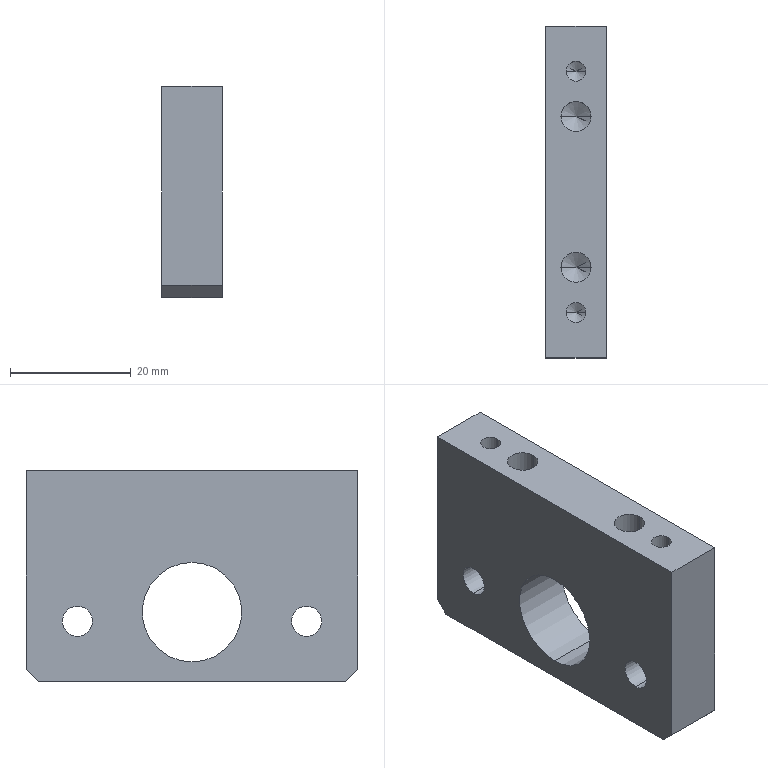Part | SolidWorks | features HoleWzd 3, Chamfer 1, Extrusion 1, ICE 1, MirrorPattern 1 | 1 solid | 30 faces | box 10 x 55 x 35 mm | volume 16084 mm3 | cylinder 14 | cone 8 | plane 8 | commonest cylinder face diameters 5 x8 3.3 x4 16.5 x2
STEP:
#1=CARTESIAN_POINT('',(2.5,12.5,7.4));
#2=VERTEX_POINT('',#1);
#3=CARTESIAN_POINT('',(7.5,12.5,7.4));
#4=VERTEX_POINT('',#3);
#5=CARTESIAN_POINT('',(5.,12.5,7.4));
#6=DIRECTION('',(0.,0.,1.));
#7=DIRECTION('',(1.,0.,0.));
#8=AXIS2_PLACEMENT_3D('',#5,#6,#7);
#9=CIRCLE('',#8,2.5);
#10=EDGE_CURVE('',#2,#4,#9,.T.);
#11=ORIENTED_EDGE('',*,*,#10,.F.);
#12=CARTESIAN_POINT('',(2.5,12.5,17.5));
#13=VERTEX_POINT('',#12);
#14=CARTESIAN_POINT('',(2.5,12.5,17.5));
#15=DIRECTION('',(0.,0.,1.));
#16=VECTOR('',#15,1000.);
#17=LINE('',#14,#16);
#18=EDGE_CURVE('',#2,#13,#17,.T.);
#19=ORIENTED_EDGE('',*,*,#18,.T.);
#20=CARTESIAN_POINT('',(7.5,12.5,17.5));
#21=VERTEX_POINT('',#20);
#22=CARTESIAN_POINT('',(5.,12.5,17.5));
#23=DIRECTION('',(0.,0.,1.));
#24=DIRECTION('',(1.,0.,0.));
#25=AXIS2_PLACEMENT_3D('',#22,#23,#24);
#26=CIRCLE('',#25,2.5);
#27=EDGE_CURVE('',#13,#21,#26,.T.);
#28=ORIENTED_EDGE('',*,*,#27,.T.);
#29=CARTESIAN_POINT('',(7.5,12.5,17.5));
#30=DIRECTION('',(0.,0.,1.));
#31=VECTOR('',#30,1000.);
#32=LINE('',#29,#31);
#33=EDGE_CURVE('',#4,#21,#32,.T.);
#34=ORIENTED_EDGE('',*,*,#33,.F.);
#35=EDGE_LOOP('',(#11,#19,#28,#34));
#36=FACE_OUTER_BOUND('',#35,.T.);
#37=CARTESIAN_POINT('',(5.,12.5,17.5));
#38=DIRECTION('',(0.,0.,1.));
#39=DIRECTION('',(1.,0.,0.));
#40=AXIS2_PLACEMENT_3D('',#37,#38,#39);
#41=CYLINDRICAL_SURFACE('',#40,2.5);
#42=ADVANCED_FACE('',(#36),#41,.F.);
#43=CARTESIAN_POINT('',(5.,12.5,5.898));
#44=VERTEX_POINT('',#43);
#45=CARTESIAN_POINT('',(7.5,12.5,7.4));
#46=DIRECTION('',(0.8572,0.,0.515));
#47=VECTOR('',#46,1000.);
#48=LINE('',#45,#47);
#49=EDGE_CURVE('',#44,#4,#48,.T.);
#50=ORIENTED_EDGE('',*,*,#49,.F.);
#51=CARTESIAN_POINT('',(2.5,12.5,7.4));
#52=DIRECTION('',(-0.8572,0.,0.515));
#53=VECTOR('',#52,1000.);
#54=LINE('',#51,#53);
#55=EDGE_CURVE('',#44,#2,#54,.T.);
#56=ORIENTED_EDGE('',*,*,#55,.T.);
#57=ORIENTED_EDGE('',*,*,#10,.T.);
#58=EDGE_LOOP('',(#50,#56,#57));
#59=FACE_OUTER_BOUND('',#58,.T.);
#60=CARTESIAN_POINT('',(5.,12.5,7.4));
#61=DIRECTION('',(0.,0.,1.));
#62=DIRECTION('',(1.,0.,0.));
#63=AXIS2_PLACEMENT_3D('',#60,#61,#62);
#64=CONICAL_SURFACE('',#63,2.5,1.03);
#65=ADVANCED_FACE('',(#59),#64,.F.);
#66=CARTESIAN_POINT('',(2.5,-12.5,7.4));
#67=VERTEX_POINT('',#66);
#68=CARTESIAN_POINT('',(7.5,-12.5,7.4));
#69=VERTEX_POINT('',#68);
#70=CARTESIAN_POINT('',(5.,-12.5,7.4));
#71=DIRECTION('',(0.,0.,1.));
#72=DIRECTION('',(1.,0.,0.));
#73=AXIS2_PLACEMENT_3D('',#70,#71,#72);
#74=CIRCLE('',#73,2.5);
#75=EDGE_CURVE('',#67,#69,#74,.T.);
#76=ORIENTED_EDGE('',*,*,#75,.F.);
#77=CARTESIAN_POINT('',(2.5,-12.5,17.5));
#78=VERTEX_POINT('',#77);
#79=CARTESIAN_POINT('',(2.5,-12.5,17.5));
#80=DIRECTION('',(0.,0.,1.));
#81=VECTOR('',#80,1000.);
#82=LINE('',#79,#81);
#83=EDGE_CURVE('',#67,#78,#82,.T.);
#84=ORIENTED_EDGE('',*,*,#83,.T.);
#85=CARTESIAN_POINT('',(7.5,-12.5,17.5));
#86=VERTEX_POINT('',#85);
#87=CARTESIAN_POINT('',(5.,-12.5,17.5));
#88=DIRECTION('',(0.,0.,1.));
#89=DIRECTION('',(1.,0.,0.));
#90=AXIS2_PLACEMENT_3D('',#87,#88,#89);
#91=CIRCLE('',#90,2.5);
#92=EDGE_CURVE('',#78,#86,#91,.T.);
#93=ORIENTED_EDGE('',*,*,#92,.T.);
#94=CARTESIAN_POINT('',(7.5,-12.5,17.5));
#95=DIRECTION('',(0.,0.,1.));
#96=VECTOR('',#95,1000.);
#97=LINE('',#94,#96);
#98=EDGE_CURVE('',#69,#86,#97,.T.);
#99=ORIENTED_EDGE('',*,*,#98,.F.);
#100=EDGE_LOOP('',(#76,#84,#93,#99));
#101=FACE_OUTER_BOUND('',#100,.T.);
#102=CARTESIAN_POINT('',(5.,-12.5,17.5));
#103=DIRECTION('',(0.,0.,1.));
#104=DIRECTION('',(1.,0.,0.));
#105=AXIS2_PLACEMENT_3D('',#102,#103,#104);
#106=CYLINDRICAL_SURFACE('',#105,2.5);
#107=ADVANCED_FACE('',(#101),#106,.F.);
#108=CARTESIAN_POINT('',(5.,-12.5,5.898));
#109=VERTEX_POINT('',#108);
#110=CARTESIAN_POINT('',(7.5,-12.5,7.4));
#111=DIRECTION('',(0.8572,0.,0.515));
#112=VECTOR('',#111,1000.);
#113=LINE('',#110,#112);
#114=EDGE_CURVE('',#109,#69,#113,.T.);
#115=ORIENTED_EDGE('',*,*,#114,.F.);
#116=CARTESIAN_POINT('',(2.5,-12.5,7.4));
#117=DIRECTION('',(-0.8572,0.,0.515));
#118=VECTOR('',#117,1000.);
#119=LINE('',#116,#118);
#120=EDGE_CURVE('',#109,#67,#119,.T.);
#121=ORIENTED_EDGE('',*,*,#120,.T.);
#122=ORIENTED_EDGE('',*,*,#75,.T.);
#123=EDGE_LOOP('',(#115,#121,#122));
#124=FACE_OUTER_BOUND('',#123,.T.);
#125=CARTESIAN_POINT('',(5.,-12.5,7.4));
#126=DIRECTION('',(0.,0.,1.));
#127=DIRECTION('',(1.,0.,0.));
#128=AXIS2_PLACEMENT_3D('',#125,#126,#127);
#129=CONICAL_SURFACE('',#128,2.5,1.03);
#130=ADVANCED_FACE('',(#124),#129,.F.);
#131=CARTESIAN_POINT('',(3.35,20.,7.4));
#132=VERTEX_POINT('',#131);
#133=CARTESIAN_POINT('',(6.65,20.,7.4));
#134=VERTEX_POINT('',#133);
#135=CARTESIAN_POINT('',(5.,20.,7.4));
#136=DIRECTION('',(0.,0.,1.));
#137=DIRECTION('',(1.,0.,0.));
#138=AXIS2_PLACEMENT_3D('',#135,#136,#137);
#139=CIRCLE('',#138,1.65);
#140=EDGE_CURVE('',#132,#134,#139,.T.);
#141=ORIENTED_EDGE('',*,*,#140,.F.);
#142=CARTESIAN_POINT('',(3.35,20.,17.5));
#143=VERTEX_POINT('',#142);
#144=CARTESIAN_POINT('',(3.35,20.,17.5));
#145=DIRECTION('',(0.,0.,1.));
#146=VECTOR('',#145,1000.);
#147=LINE('',#144,#146);
#148=EDGE_CURVE('',#132,#143,#147,.T.);
#149=ORIENTED_EDGE('',*,*,#148,.T.);
#150=CARTESIAN_POINT('',(6.65,20.,17.5));
#151=VERTEX_POINT('',#150);
#152=CARTESIAN_POINT('',(5.,20.,17.5));
#153=DIRECTION('',(0.,0.,1.));
#154=DIRECTION('',(1.,0.,0.));
#155=AXIS2_PLACEMENT_3D('',#152,#153,#154);
#156=CIRCLE('',#155,1.65);
#157=EDGE_CURVE('',#143,#151,#156,.T.);
#158=ORIENTED_EDGE('',*,*,#157,.T.);
#159=CARTESIAN_POINT('',(6.65,20.,17.5));
#160=DIRECTION('',(0.,0.,1.));
#161=VECTOR('',#160,1000.);
#162=LINE('',#159,#161);
#163=EDGE_CURVE('',#134,#151,#162,.T.);
#164=ORIENTED_EDGE('',*,*,#163,.F.);
#165=EDGE_LOOP('',(#141,#149,#158,#164));
#166=FACE_OUTER_BOUND('',#165,.T.);
#167=CARTESIAN_POINT('',(5.,20.,17.5));
#168=DIRECTION('',(0.,0.,1.));
#169=DIRECTION('',(1.,0.,0.));
#170=AXIS2_PLACEMENT_3D('',#167,#168,#169);
#171=CYLINDRICAL_SURFACE('',#170,1.65);
#172=ADVANCED_FACE('',(#166),#171,.F.);
#173=CARTESIAN_POINT('',(5.,20.,6.409));
#174=VERTEX_POINT('',#173);
#175=CARTESIAN_POINT('',(6.65,20.,7.4));
#176=DIRECTION('',(0.8572,0.,0.515));
#177=VECTOR('',#176,1000.);
#178=LINE('',#175,#177);
#179=EDGE_CURVE('',#174,#134,#178,.T.);
#180=ORIENTED_EDGE('',*,*,#179,.F.);
#181=CARTESIAN_POINT('',(3.35,20.,7.4));
#182=DIRECTION('',(-0.8572,0.,0.515));
#183=VECTOR('',#182,1000.);
#184=LINE('',#181,#183);
#185=EDGE_CURVE('',#174,#132,#184,.T.);
#186=ORIENTED_EDGE('',*,*,#185,.T.);
#187=ORIENTED_EDGE('',*,*,#140,.T.);
#188=EDGE_LOOP('',(#180,#186,#187));
#189=FACE_OUTER_BOUND('',#188,.T.);
#190=CARTESIAN_POINT('',(5.,20.,7.4));
#191=DIRECTION('',(0.,0.,1.));
#192=DIRECTION('',(1.,0.,0.));
#193=AXIS2_PLACEMENT_3D('',#190,#191,#192);
#194=CONICAL_SURFACE('',#193,1.65,1.03);
#195=ADVANCED_FACE('',(#189),#194,.F.);
#196=CARTESIAN_POINT('',(3.35,-20.,7.4));
#197=VERTEX_POINT('',#196);
#198=CARTESIAN_POINT('',(6.65,-20.,7.4));
#199=VERTEX_POINT('',#198);
#200=CARTESIAN_POINT('',(5.,-20.,7.4));
#201=DIRECTION('',(0.,0.,1.));
#202=DIRECTION('',(1.,0.,0.));
#203=AXIS2_PLACEMENT_3D('',#200,#201,#202);
#204=CIRCLE('',#203,1.65);
#205=EDGE_CURVE('',#197,#199,#204,.T.);
#206=ORIENTED_EDGE('',*,*,#205,.F.);
#207=CARTESIAN_POINT('',(3.35,-20.,17.5));
#208=VERTEX_POINT('',#207);
#209=CARTESIAN_POINT('',(3.35,-20.,17.5));
#210=DIRECTION('',(0.,0.,1.));
#211=VECTOR('',#210,1000.);
#212=LINE('',#209,#211);
#213=EDGE_CURVE('',#197,#208,#212,.T.);
#214=ORIENTED_EDGE('',*,*,#213,.T.);
#215=CARTESIAN_POINT('',(6.65,-20.,17.5));
#216=VERTEX_POINT('',#215);
#217=CARTESIAN_POINT('',(5.,-20.,17.5));
#218=DIRECTION('',(0.,0.,1.));
#219=DIRECTION('',(1.,0.,0.));
#220=AXIS2_PLACEMENT_3D('',#217,#218,#219);
#221=CIRCLE('',#220,1.65);
#222=EDGE_CURVE('',#208,#216,#221,.T.);
#223=ORIENTED_EDGE('',*,*,#222,.T.);
#224=CARTESIAN_POINT('',(6.65,-20.,17.5));
#225=DIRECTION('',(0.,0.,1.));
#226=VECTOR('',#225,1000.);
#227=LINE('',#224,#226);
#228=EDGE_CURVE('',#199,#216,#227,.T.);
#229=ORIENTED_EDGE('',*,*,#228,.F.);
#230=EDGE_LOOP('',(#206,#214,#223,#229));
#231=FACE_OUTER_BOUND('',#230,.T.);
#232=CARTESIAN_POINT('',(5.,-20.,17.5));
#233=DIRECTION('',(0.,0.,1.));
#234=DIRECTION('',(1.,0.,0.));
#235=AXIS2_PLACEMENT_3D('',#232,#233,#234);
#236=CYLINDRICAL_SURFACE('',#235,1.65);
#237=ADVANCED_FACE('',(#231),#236,.F.);
#238=CARTESIAN_POINT('',(5.,-20.,6.409));
#239=VERTEX_POINT('',#238);
#240=CARTESIAN_POINT('',(6.65,-20.,7.4));
#241=DIRECTION('',(0.8572,0.,0.515));
#242=VECTOR('',#241,1000.);
#243=LINE('',#240,#242);
#244=EDGE_CURVE('',#239,#199,#243,.T.);
#245=ORIENTED_EDGE('',*,*,#244,.F.);
#246=CARTESIAN_POINT('',(3.35,-20.,7.4));
#247=DIRECTION('',(-0.8572,0.,0.515));
#248=VECTOR('',#247,1000.);
#249=LINE('',#246,#248);
#250=EDGE_CURVE('',#239,#197,#249,.T.);
#251=ORIENTED_EDGE('',*,*,#250,.T.);
#252=ORIENTED_EDGE('',*,*,#205,.T.);
#253=EDGE_LOOP('',(#245,#251,#252));
#254=FACE_OUTER_BOUND('',#253,.T.);
#255=CARTESIAN_POINT('',(5.,-20.,7.4));
#256=DIRECTION('',(0.,0.,1.));
#257=DIRECTION('',(1.,0.,0.));
#258=AXIS2_PLACEMENT_3D('',#255,#256,#257);
#259=CONICAL_SURFACE('',#258,1.65,1.03);
#260=ADVANCED_FACE('',(#254),#259,.F.);
#261=CARTESIAN_POINT('',(10.,19.,-10.));
#262=VERTEX_POINT('',#261);
#263=CARTESIAN_POINT('',(10.,19.,-5.));
#264=VERTEX_POINT('',#263);
#265=CARTESIAN_POINT('',(10.,19.,-7.5));
#266=DIRECTION('',(-1.,0.,0.));
#267=DIRECTION('',(0.,0.,1.));
#268=AXIS2_PLACEMENT_3D('',#265,#266,#267);
#269=CIRCLE('',#268,2.5);
#270=EDGE_CURVE('',#262,#264,#269,.T.);
#271=ORIENTED_EDGE('',*,*,#270,.F.);
#272=CARTESIAN_POINT('',(0.,19.,-10.));
#273=VERTEX_POINT('',#272);
#274=CARTESIAN_POINT('',(0.,19.,-10.));
#275=DIRECTION('',(-1.,0.,0.));
#276=VECTOR('',#275,1000.);
#277=LINE('',#274,#276);
#278=EDGE_CURVE('',#262,#273,#277,.T.);
#279=ORIENTED_EDGE('',*,*,#278,.T.);
#280=CARTESIAN_POINT('',(0.,19.,-5.));
#281=VERTEX_POINT('',#280);
#282=CARTESIAN_POINT('',(0.,19.,-7.5));
#283=DIRECTION('',(-1.,0.,0.));
#284=DIRECTION('',(0.,0.,1.));
#285=AXIS2_PLACEMENT_3D('',#282,#283,#284);
#286=CIRCLE('',#285,2.5);
#287=EDGE_CURVE('',#273,#281,#286,.T.);
#288=ORIENTED_EDGE('',*,*,#287,.T.);
#289=CARTESIAN_POINT('',(0.,19.,-5.));
#290=DIRECTION('',(-1.,0.,0.));
#291=VECTOR('',#290,1000.);
#292=LINE('',#289,#291);
#293=EDGE_CURVE('',#264,#281,#292,.T.);
#294=ORIENTED_EDGE('',*,*,#293,.F.);
#295=EDGE_LOOP('',(#271,#279,#288,#294));
#296=FACE_OUTER_BOUND('',#295,.T.);
#297=CARTESIAN_POINT('',(0.,19.,-7.5));
#298=DIRECTION('',(-1.,0.,0.));
#299=DIRECTION('',(0.,0.,1.));
#300=AXIS2_PLACEMENT_3D('',#297,#298,#299);
#301=CYLINDRICAL_SURFACE('',#300,2.5);
#302=ADVANCED_FACE('',(#296),#301,.F.);
#303=CARTESIAN_POINT('',(10.,-19.,-10.));
#304=VERTEX_POINT('',#303);
#305=CARTESIAN_POINT('',(10.,-19.,-5.));
#306=VERTEX_POINT('',#305);
#307=CARTESIAN_POINT('',(10.,-19.,-7.5));
#308=DIRECTION('',(-1.,0.,0.));
#309=DIRECTION('',(0.,0.,1.));
#310=AXIS2_PLACEMENT_3D('',#307,#308,#309);
#311=CIRCLE('',#310,2.5);
#312=EDGE_CURVE('',#304,#306,#311,.T.);
#313=ORIENTED_EDGE('',*,*,#312,.F.);
#314=CARTESIAN_POINT('',(0.,-19.,-10.));
#315=VERTEX_POINT('',#314);
#316=CARTESIAN_POINT('',(0.,-19.,-10.));
#317=DIRECTION('',(-1.,0.,0.));
#318=VECTOR('',#317,1000.);
#319=LINE('',#316,#318);
#320=EDGE_CURVE('',#304,#315,#319,.T.);
#321=ORIENTED_EDGE('',*,*,#320,.T.);
#322=CARTESIAN_POINT('',(0.,-19.,-5.));
#323=VERTEX_POINT('',#322);
#324=CARTESIAN_POINT('',(0.,-19.,-7.5));
#325=DIRECTION('',(-1.,0.,0.));
#326=DIRECTION('',(0.,0.,1.));
#327=AXIS2_PLACEMENT_3D('',#324,#325,#326);
#328=CIRCLE('',#327,2.5);
#329=EDGE_CURVE('',#315,#323,#328,.T.);
#330=ORIENTED_EDGE('',*,*,#329,.T.);
#331=CARTESIAN_POINT('',(0.,-19.,-5.));
#332=DIRECTION('',(-1.,0.,0.));
#333=VECTOR('',#332,1000.);
#334=LINE('',#331,#333);
#335=EDGE_CURVE('',#306,#323,#334,.T.);
#336=ORIENTED_EDGE('',*,*,#335,.F.);
#337=EDGE_LOOP('',(#313,#321,#330,#336));
#338=FACE_OUTER_BOUND('',#337,.T.);
#339=CARTESIAN_POINT('',(0.,-19.,-7.5));
#340=DIRECTION('',(-1.,0.,0.));
#341=DIRECTION('',(0.,0.,1.));
#342=AXIS2_PLACEMENT_3D('',#339,#340,#341);
#343=CYLINDRICAL_SURFACE('',#342,2.5);
#344=ADVANCED_FACE('',(#338),#343,.F.);
#345=CARTESIAN_POINT('',(10.,0.,2.25));
#346=VERTEX_POINT('',#345);
#347=CARTESIAN_POINT('',(10.,0.,-14.25));
#348=VERTEX_POINT('',#347);
#349=CARTESIAN_POINT('',(10.,0.,-6.));
#350=DIRECTION('',(1.,0.,0.));
#351=DIRECTION('',(0.,0.,-1.));
#352=AXIS2_PLACEMENT_3D('',#349,#350,#351);
#353=CIRCLE('',#352,8.25);
#354=EDGE_CURVE('',#346,#348,#353,.T.);
#355=ORIENTED_EDGE('',*,*,#354,.T.);
#356=CARTESIAN_POINT('',(0.,0.,-14.25));
#357=VERTEX_POINT('',#356);
#358=CARTESIAN_POINT('',(110.,0.,-14.25));
#359=DIRECTION('',(-1.,0.,0.));
#360=VECTOR('',#359,1000.);
#361=LINE('',#358,#360);
#362=EDGE_CURVE('',#348,#357,#361,.T.);
#363=ORIENTED_EDGE('',*,*,#362,.T.);
#364=CARTESIAN_POINT('',(0.,0.,2.25));
#365=VERTEX_POINT('',#364);
#366=CARTESIAN_POINT('',(0.,0.,-6.));
#367=DIRECTION('',(-1.,0.,0.));
#368=DIRECTION('',(0.,0.,1.));
#369=AXIS2_PLACEMENT_3D('',#366,#367,#368);
#370=CIRCLE('',#369,8.25);
#371=EDGE_CURVE('',#357,#365,#370,.T.);
#372=ORIENTED_EDGE('',*,*,#371,.T.);
#373=CARTESIAN_POINT('',(110.,0.,2.25));
#374=DIRECTION('',(-1.,0.,0.));
#375=VECTOR('',#374,1000.);
#376=LINE('',#373,#375);
#377=EDGE_CURVE('',#346,#365,#376,.T.);
#378=ORIENTED_EDGE('',*,*,#377,.F.);
#379=EDGE_LOOP('',(#355,#363,#372,#378));
#380=FACE_OUTER_BOUND('',#379,.T.);
#381=CARTESIAN_POINT('',(110.,0.,-6.));
#382=DIRECTION('',(-1.,0.,0.));
#383=DIRECTION('',(0.,0.,1.));
#384=AXIS2_PLACEMENT_3D('',#381,#382,#383);
#385=CYLINDRICAL_SURFACE('',#384,8.25);
#386=ADVANCED_FACE('',(#380),#385,.F.);
#387=CARTESIAN_POINT('',(10.,-25.5,-17.5));
#388=VERTEX_POINT('',#387);
#389=CARTESIAN_POINT('',(10.,25.5,-17.5));
#390=VERTEX_POINT('',#389);
#391=CARTESIAN_POINT('',(10.,27.5,-17.5));
#392=DIRECTION('',(0.,1.,0.));
#393=VECTOR('',#392,1000.);
#394=LINE('',#391,#393);
#395=EDGE_CURVE('',#388,#390,#394,.T.);
#396=ORIENTED_EDGE('',*,*,#395,.F.);
#397=CARTESIAN_POINT('',(0.,-25.5,-17.5));
#398=VERTEX_POINT('',#397);
#399=CARTESIAN_POINT('',(10.,-25.5,-17.5));
#400=DIRECTION('',(-1.,0.,0.));
#401=VECTOR('',#400,1000.);
#402=LINE('',#399,#401);
#403=EDGE_CURVE('',#388,#398,#402,.T.);
#404=ORIENTED_EDGE('',*,*,#403,.T.);
#405=CARTESIAN_POINT('',(0.,25.5,-17.5));
#406=VERTEX_POINT('',#405);
#407=CARTESIAN_POINT('',(0.,27.5,-17.5));
#408=DIRECTION('',(0.,1.,0.));
#409=VECTOR('',#408,1000.);
#410=LINE('',#407,#409);
#411=EDGE_CURVE('',#398,#406,#410,.T.);
#412=ORIENTED_EDGE('',*,*,#411,.T.);
#413=CARTESIAN_POINT('',(10.,25.5,-17.5));
#414=DIRECTION('',(1.,0.,0.));
#415=VECTOR('',#414,1000.);
#416=LINE('',#413,#415);
#417=EDGE_CURVE('',#406,#390,#416,.T.);
#418=ORIENTED_EDGE('',*,*,#417,.T.);
#419=EDGE_LOOP('',(#396,#404,#412,#418));
#420=FACE_OUTER_BOUND('',#419,.T.);
#421=CARTESIAN_POINT('',(10.,27.5,-17.5));
#422=DIRECTION('',(0.,0.,1.));
#423=DIRECTION('',(0.,-1.,0.));
#424=AXIS2_PLACEMENT_3D('',#421,#422,#423);
#425=PLANE('',#424);
#426=ADVANCED_FACE('',(#420),#425,.F.);
#427=CARTESIAN_POINT('',(10.,27.5,-15.5));
#428=VERTEX_POINT('',#427);
#429=CARTESIAN_POINT('',(10.,27.5,17.5));
#430=VERTEX_POINT('',#429);
#431=CARTESIAN_POINT('',(10.,27.5,17.5));
#432=DIRECTION('',(0.,0.,1.));
#433=VECTOR('',#432,1000.);
#434=LINE('',#431,#433);
#435=EDGE_CURVE('',#428,#430,#434,.T.);
#436=ORIENTED_EDGE('',*,*,#435,.F.);
#437=CARTESIAN_POINT('',(0.,27.5,-15.5));
#438=VERTEX_POINT('',#437);
#439=CARTESIAN_POINT('',(10.,27.5,-15.5));
#440=DIRECTION('',(-1.,0.,0.));
#441=VECTOR('',#440,1000.);
#442=LINE('',#439,#441);
#443=EDGE_CURVE('',#428,#438,#442,.T.);
#444=ORIENTED_EDGE('',*,*,#443,.T.);
#445=CARTESIAN_POINT('',(0.,27.5,17.5));
#446=VERTEX_POINT('',#445);
#447=CARTESIAN_POINT('',(0.,27.5,17.5));
#448=DIRECTION('',(0.,0.,1.));
#449=VECTOR('',#448,1000.);
#450=LINE('',#447,#449);
#451=EDGE_CURVE('',#438,#446,#450,.T.);
#452=ORIENTED_EDGE('',*,*,#451,.T.);
#453=CARTESIAN_POINT('',(10.,27.5,17.5));
#454=DIRECTION('',(-1.,0.,0.));
#455=VECTOR('',#454,1000.);
#456=LINE('',#453,#455);
#457=EDGE_CURVE('',#430,#446,#456,.T.);
#458=ORIENTED_EDGE('',*,*,#457,.F.);
#459=EDGE_LOOP('',(#436,#444,#452,#458));
#460=FACE_OUTER_BOUND('',#459,.T.);
#461=CARTESIAN_POINT('',(10.,27.5,17.5));
#462=DIRECTION('',(0.,-1.,0.));
#463=DIRECTION('',(0.,0.,-1.));
#464=AXIS2_PLACEMENT_3D('',#461,#462,#463);
#465=PLANE('',#464);
#466=ADVANCED_FACE('',(#460),#465,.F.);
#467=CARTESIAN_POINT('',(5.,12.5,17.5));
#468=DIRECTION('',(0.,0.,1.));
#469=DIRECTION('',(1.,0.,0.));
#470=AXIS2_PLACEMENT_3D('',#467,#468,#469);
#471=CIRCLE('',#470,2.5);
#472=EDGE_CURVE('',#21,#13,#471,.T.);
#473=ORIENTED_EDGE('',*,*,#472,.F.);
#474=ORIENTED_EDGE('',*,*,#27,.F.);
#475=EDGE_LOOP('',(#473,#474));
#476=FACE_BOUND('',#475,.T.);
#477=CARTESIAN_POINT('',(5.,-12.5,17.5));
#478=DIRECTION('',(0.,0.,1.));
#479=DIRECTION('',(1.,0.,0.));
#480=AXIS2_PLACEMENT_3D('',#477,#478,#479);
#481=CIRCLE('',#480,2.5);
#482=EDGE_CURVE('',#86,#78,#481,.T.);
#483=ORIENTED_EDGE('',*,*,#482,.F.);
#484=ORIENTED_EDGE('',*,*,#92,.F.);
#485=EDGE_LOOP('',(#483,#484));
#486=FACE_BOUND('',#485,.T.);
#487=CARTESIAN_POINT('',(5.,20.,17.5));
#488=DIRECTION('',(0.,0.,1.));
#489=DIRECTION('',(1.,0.,0.));
#490=AXIS2_PLACEMENT_3D('',#487,#488,#489);
#491=CIRCLE('',#490,1.65);
#492=EDGE_CURVE('',#151,#143,#491,.T.);
#493=ORIENTED_EDGE('',*,*,#492,.F.);
#494=ORIENTED_EDGE('',*,*,#157,.F.);
#495=EDGE_LOOP('',(#493,#494));
#496=FACE_BOUND('',#495,.T.);
#497=CARTESIAN_POINT('',(5.,-20.,17.5));
#498=DIRECTION('',(0.,0.,1.));
#499=DIRECTION('',(1.,0.,0.));
#500=AXIS2_PLACEMENT_3D('',#497,#498,#499);
#501=CIRCLE('',#500,1.65);
#502=EDGE_CURVE('',#216,#208,#501,.T.);
#503=ORIENTED_EDGE('',*,*,#502,.F.);
#504=ORIENTED_EDGE('',*,*,#222,.F.);
#505=EDGE_LOOP('',(#503,#504));
#506=FACE_BOUND('',#505,.T.);
#507=CARTESIAN_POINT('',(0.,-27.5,17.5));
#508=VERTEX_POINT('',#507);
#509=CARTESIAN_POINT('',(0.,27.5,17.5));
#510=DIRECTION('',(0.,-1.,0.));
#511=VECTOR('',#510,1000.);
#512=LINE('',#509,#511);
#513=EDGE_CURVE('',#446,#508,#512,.T.);
#514=ORIENTED_EDGE('',*,*,#513,.T.);
#515=CARTESIAN_POINT('',(10.,-27.5,17.5));
#516=VERTEX_POINT('',#515);
#517=CARTESIAN_POINT('',(10.,-27.5,17.5));
#518=DIRECTION('',(-1.,0.,0.));
#519=VECTOR('',#518,1000.);
#520=LINE('',#517,#519);
#521=EDGE_CURVE('',#516,#508,#520,.T.);
#522=ORIENTED_EDGE('',*,*,#521,.F.);
#523=CARTESIAN_POINT('',(10.,27.5,17.5));
#524=DIRECTION('',(0.,-1.,0.));
#525=VECTOR('',#524,1000.);
#526=LINE('',#523,#525);
#527=EDGE_CURVE('',#430,#516,#526,.T.);
#528=ORIENTED_EDGE('',*,*,#527,.F.);
#529=ORIENTED_EDGE('',*,*,#457,.T.);
#530=EDGE_LOOP('',(#514,#522,#528,#529));
#531=FACE_OUTER_BOUND('',#530,.T.);
#532=CARTESIAN_POINT('',(10.,27.5,17.5));
#533=DIRECTION('',(0.,0.,-1.));
#534=DIRECTION('',(0.,1.,0.));
#535=AXIS2_PLACEMENT_3D('',#532,#533,#534);
#536=PLANE('',#535);
#537=ADVANCED_FACE('',(#476,#486,#496,#506,#531),#536,.F.);
#538=CARTESIAN_POINT('',(0.,-27.5,-15.5));
#539=VERTEX_POINT('',#538);
#540=CARTESIAN_POINT('',(0.,-27.5,17.5));
#541=DIRECTION('',(0.,0.,-1.));
#542=VECTOR('',#541,1000.);
#543=LINE('',#540,#542);
#544=EDGE_CURVE('',#508,#539,#543,.T.);
#545=ORIENTED_EDGE('',*,*,#544,.T.);
#546=CARTESIAN_POINT('',(10.,-27.5,-15.5));
#547=VERTEX_POINT('',#546);
#548=CARTESIAN_POINT('',(10.,-27.5,-15.5));
#549=DIRECTION('',(1.,0.,0.));
#550=VECTOR('',#549,1000.);
#551=LINE('',#548,#550);
#552=EDGE_CURVE('',#539,#547,#551,.T.);
#553=ORIENTED_EDGE('',*,*,#552,.T.);
#554=CARTESIAN_POINT('',(10.,-27.5,17.5));
#555=DIRECTION('',(0.,0.,-1.));
#556=VECTOR('',#555,1000.);
#557=LINE('',#554,#556);
#558=EDGE_CURVE('',#516,#547,#557,.T.);
#559=ORIENTED_EDGE('',*,*,#558,.F.);
#560=ORIENTED_EDGE('',*,*,#521,.T.);
#561=EDGE_LOOP('',(#545,#553,#559,#560));
#562=FACE_OUTER_BOUND('',#561,.T.);
#563=CARTESIAN_POINT('',(10.,-27.5,17.5));
#564=DIRECTION('',(0.,1.,0.));
#565=DIRECTION('',(0.,0.,1.));
#566=AXIS2_PLACEMENT_3D('',#563,#564,#565);
#567=PLANE('',#566);
#568=ADVANCED_FACE('',(#562),#567,.F.);
#569=CARTESIAN_POINT('',(10.,19.,-7.5));
#570=DIRECTION('',(-1.,0.,0.));
#571=DIRECTION('',(0.,0.,1.));
#572=AXIS2_PLACEMENT_3D('',#569,#570,#571);
#573=CIRCLE('',#572,2.5);
#574=EDGE_CURVE('',#264,#262,#573,.T.);
#575=ORIENTED_EDGE('',*,*,#574,.T.);
#576=ORIENTED_EDGE('',*,*,#270,.T.);
#577=EDGE_LOOP('',(#575,#576));
#578=FACE_BOUND('',#577,.T.);
#579=CARTESIAN_POINT('',(10.,-19.,-7.5));
#580=DIRECTION('',(-1.,0.,0.));
#581=DIRECTION('',(0.,0.,1.));
#582=AXIS2_PLACEMENT_3D('',#579,#580,#581);
#583=CIRCLE('',#582,2.5);
#584=EDGE_CURVE('',#306,#304,#583,.T.);
#585=ORIENTED_EDGE('',*,*,#584,.T.);
#586=ORIENTED_EDGE('',*,*,#312,.T.);
#587=EDGE_LOOP('',(#585,#586));
#588=FACE_BOUND('',#587,.T.);
#589=ORIENTED_EDGE('',*,*,#354,.F.);
#590=CARTESIAN_POINT('',(10.,0.,-6.));
#591=DIRECTION('',(1.,0.,0.));
#592=DIRECTION('',(0.,0.,-1.));
#593=AXIS2_PLACEMENT_3D('',#590,#591,#592);
#594=CIRCLE('',#593,8.25);
#595=EDGE_CURVE('',#348,#346,#594,.T.);
#596=ORIENTED_EDGE('',*,*,#595,.F.);
#597=EDGE_LOOP('',(#589,#596));
#598=FACE_BOUND('',#597,.T.);
#599=ORIENTED_EDGE('',*,*,#558,.T.);
#600=CARTESIAN_POINT('',(10.,-21.5,-21.5));
#601=DIRECTION('',(0.,0.7071,-0.7071));
#602=VECTOR('',#601,1000.);
#603=LINE('',#600,#602);
#604=EDGE_CURVE('',#547,#388,#603,.T.);
#605=ORIENTED_EDGE('',*,*,#604,.T.);
#606=ORIENTED_EDGE('',*,*,#395,.T.);
#607=CARTESIAN_POINT('',(10.,21.5,-21.5));
#608=DIRECTION('',(0.,0.7071,0.7071));
#609=VECTOR('',#608,1000.);
#610=LINE('',#607,#609);
#611=EDGE_CURVE('',#390,#428,#610,.T.);
#612=ORIENTED_EDGE('',*,*,#611,.T.);
#613=ORIENTED_EDGE('',*,*,#435,.T.);
#614=ORIENTED_EDGE('',*,*,#527,.T.);
#615=EDGE_LOOP('',(#599,#605,#606,#612,#613,#614));
#616=FACE_OUTER_BOUND('',#615,.T.);
#617=CARTESIAN_POINT('',(10.,0.,0.));
#618=DIRECTION('',(1.,0.,0.));
#619=DIRECTION('',(0.,0.,-1.));
#620=AXIS2_PLACEMENT_3D('',#617,#618,#619);
#621=PLANE('',#620);
#622=ADVANCED_FACE('',(#578,#588,#598,#616),#621,.T.);
#623=CARTESIAN_POINT('',(0.,19.,-7.5));
#624=DIRECTION('',(-1.,0.,0.));
#625=DIRECTION('',(0.,0.,1.));
#626=AXIS2_PLACEMENT_3D('',#623,#624,#625);
#627=CIRCLE('',#626,2.5);
#628=EDGE_CURVE('',#281,#273,#627,.T.);
#629=ORIENTED_EDGE('',*,*,#628,.F.);
#630=ORIENTED_EDGE('',*,*,#287,.F.);
#631=EDGE_LOOP('',(#629,#630));
#632=FACE_BOUND('',#631,.T.);
#633=CARTESIAN_POINT('',(0.,-19.,-7.5));
#634=DIRECTION('',(-1.,0.,0.));
#635=DIRECTION('',(0.,0.,1.));
#636=AXIS2_PLACEMENT_3D('',#633,#634,#635);
#637=CIRCLE('',#636,2.5);
#638=EDGE_CURVE('',#323,#315,#637,.T.);
#639=ORIENTED_EDGE('',*,*,#638,.F.);
#640=ORIENTED_EDGE('',*,*,#329,.F.);
#641=EDGE_LOOP('',(#639,#640));
#642=FACE_BOUND('',#641,.T.);
#643=CARTESIAN_POINT('',(0.,0.,-6.));
#644=DIRECTION('',(-1.,0.,0.));
#645=DIRECTION('',(0.,0.,1.));
#646=AXIS2_PLACEMENT_3D('',#643,#644,#645);
#647=CIRCLE('',#646,8.25);
#648=EDGE_CURVE('',#365,#357,#647,.T.);
#649=ORIENTED_EDGE('',*,*,#648,.F.);
#650=ORIENTED_EDGE('',*,*,#371,.F.);
#651=EDGE_LOOP('',(#649,#650));
#652=FACE_BOUND('',#651,.T.);
#653=ORIENTED_EDGE('',*,*,#411,.F.);
#654=CARTESIAN_POINT('',(0.,-25.5,-17.5));
#655=DIRECTION('',(0.,-0.7071,0.7071));
#656=VECTOR('',#655,1000.);
#657=LINE('',#654,#656);
#658=EDGE_CURVE('',#398,#539,#657,.T.);
#659=ORIENTED_EDGE('',*,*,#658,.T.);
#660=ORIENTED_EDGE('',*,*,#544,.F.);
#661=ORIENTED_EDGE('',*,*,#513,.F.);
#662=ORIENTED_EDGE('',*,*,#451,.F.);
#663=CARTESIAN_POINT('',(0.,27.5,-15.5));
#664=DIRECTION('',(0.,-0.7071,-0.7071));
#665=VECTOR('',#664,1000.);
#666=LINE('',#663,#665);
#667=EDGE_CURVE('',#438,#406,#666,.T.);
#668=ORIENTED_EDGE('',*,*,#667,.T.);
#669=EDGE_LOOP('',(#653,#659,#660,#661,#662,#668));
#670=FACE_OUTER_BOUND('',#669,.T.);
#671=CARTESIAN_POINT('',(0.,0.,0.));
#672=DIRECTION('',(1.,0.,0.));
#673=DIRECTION('',(0.,0.,-1.));
#674=AXIS2_PLACEMENT_3D('',#671,#672,#673);
#675=PLANE('',#674);
#676=ADVANCED_FACE('',(#632,#642,#652,#670),#675,.F.);
#677=ORIENTED_EDGE('',*,*,#362,.F.);
#678=ORIENTED_EDGE('',*,*,#595,.T.);
#679=ORIENTED_EDGE('',*,*,#377,.T.);
#680=ORIENTED_EDGE('',*,*,#648,.T.);
#681=EDGE_LOOP('',(#677,#678,#679,#680));
#682=FACE_OUTER_BOUND('',#681,.T.);
#683=CARTESIAN_POINT('',(110.,0.,-6.));
#684=DIRECTION('',(-1.,0.,0.));
#685=DIRECTION('',(0.,0.,1.));
#686=AXIS2_PLACEMENT_3D('',#683,#684,#685);
#687=CYLINDRICAL_SURFACE('',#686,8.25);
#688=ADVANCED_FACE('',(#682),#687,.F.);
#689=ORIENTED_EDGE('',*,*,#320,.F.);
#690=ORIENTED_EDGE('',*,*,#584,.F.);
#691=ORIENTED_EDGE('',*,*,#335,.T.);
#692=ORIENTED_EDGE('',*,*,#638,.T.);
#693=EDGE_LOOP('',(#689,#690,#691,#692));
#694=FACE_OUTER_BOUND('',#693,.T.);
#695=CARTESIAN_POINT('',(0.,-19.,-7.5));
#696=DIRECTION('',(-1.,0.,0.));
#697=DIRECTION('',(0.,0.,1.));
#698=AXIS2_PLACEMENT_3D('',#695,#696,#697);
#699=CYLINDRICAL_SURFACE('',#698,2.5);
#700=ADVANCED_FACE('',(#694),#699,.F.);
#701=ORIENTED_EDGE('',*,*,#278,.F.);
#702=ORIENTED_EDGE('',*,*,#574,.F.);
#703=ORIENTED_EDGE('',*,*,#293,.T.);
#704=ORIENTED_EDGE('',*,*,#628,.T.);
#705=EDGE_LOOP('',(#701,#702,#703,#704));
#706=FACE_OUTER_BOUND('',#705,.T.);
#707=CARTESIAN_POINT('',(0.,19.,-7.5));
#708=DIRECTION('',(-1.,0.,0.));
#709=DIRECTION('',(0.,0.,1.));
#710=AXIS2_PLACEMENT_3D('',#707,#708,#709);
#711=CYLINDRICAL_SURFACE('',#710,2.5);
#712=ADVANCED_FACE('',(#706),#711,.F.);
#713=ORIENTED_EDGE('',*,*,#250,.F.);
#714=ORIENTED_EDGE('',*,*,#244,.T.);
#715=CARTESIAN_POINT('',(5.,-20.,7.4));
#716=DIRECTION('',(0.,0.,1.));
#717=DIRECTION('',(1.,0.,0.));
#718=AXIS2_PLACEMENT_3D('',#715,#716,#717);
#719=CIRCLE('',#718,1.65);
#720=EDGE_CURVE('',#199,#197,#719,.T.);
#721=ORIENTED_EDGE('',*,*,#720,.T.);
#722=EDGE_LOOP('',(#713,#714,#721));
#723=FACE_OUTER_BOUND('',#722,.T.);
#724=CARTESIAN_POINT('',(5.,-20.,7.4));
#725=DIRECTION('',(0.,0.,1.));
#726=DIRECTION('',(1.,0.,0.));
#727=AXIS2_PLACEMENT_3D('',#724,#725,#726);
#728=CONICAL_SURFACE('',#727,1.65,1.03);
#729=ADVANCED_FACE('',(#723),#728,.F.);
#730=ORIENTED_EDGE('',*,*,#213,.F.);
#731=ORIENTED_EDGE('',*,*,#720,.F.);
#732=ORIENTED_EDGE('',*,*,#228,.T.);
#733=ORIENTED_EDGE('',*,*,#502,.T.);
#734=EDGE_LOOP('',(#730,#731,#732,#733));
#735=FACE_OUTER_BOUND('',#734,.T.);
#736=CARTESIAN_POINT('',(5.,-20.,17.5));
#737=DIRECTION('',(0.,0.,1.));
#738=DIRECTION('',(1.,0.,0.));
#739=AXIS2_PLACEMENT_3D('',#736,#737,#738);
#740=CYLINDRICAL_SURFACE('',#739,1.65);
#741=ADVANCED_FACE('',(#735),#740,.F.);
#742=ORIENTED_EDGE('',*,*,#185,.F.);
#743=ORIENTED_EDGE('',*,*,#179,.T.);
#744=CARTESIAN_POINT('',(5.,20.,7.4));
#745=DIRECTION('',(0.,0.,1.));
#746=DIRECTION('',(1.,0.,0.));
#747=AXIS2_PLACEMENT_3D('',#744,#745,#746);
#748=CIRCLE('',#747,1.65);
#749=EDGE_CURVE('',#134,#132,#748,.T.);
#750=ORIENTED_EDGE('',*,*,#749,.T.);
#751=EDGE_LOOP('',(#742,#743,#750));
#752=FACE_OUTER_BOUND('',#751,.T.);
#753=CARTESIAN_POINT('',(5.,20.,7.4));
#754=DIRECTION('',(0.,0.,1.));
#755=DIRECTION('',(1.,0.,0.));
#756=AXIS2_PLACEMENT_3D('',#753,#754,#755);
#757=CONICAL_SURFACE('',#756,1.65,1.03);
#758=ADVANCED_FACE('',(#752),#757,.F.);
#759=ORIENTED_EDGE('',*,*,#148,.F.);
#760=ORIENTED_EDGE('',*,*,#749,.F.);
#761=ORIENTED_EDGE('',*,*,#163,.T.);
#762=ORIENTED_EDGE('',*,*,#492,.T.);
#763=EDGE_LOOP('',(#759,#760,#761,#762));
#764=FACE_OUTER_BOUND('',#763,.T.);
#765=CARTESIAN_POINT('',(5.,20.,17.5));
#766=DIRECTION('',(0.,0.,1.));
#767=DIRECTION('',(1.,0.,0.));
#768=AXIS2_PLACEMENT_3D('',#765,#766,#767);
#769=CYLINDRICAL_SURFACE('',#768,1.65);
#770=ADVANCED_FACE('',(#764),#769,.F.);
#771=ORIENTED_EDGE('',*,*,#120,.F.);
#772=ORIENTED_EDGE('',*,*,#114,.T.);
#773=CARTESIAN_POINT('',(5.,-12.5,7.4));
#774=DIRECTION('',(0.,0.,1.));
#775=DIRECTION('',(1.,0.,0.));
#776=AXIS2_PLACEMENT_3D('',#773,#774,#775);
#777=CIRCLE('',#776,2.5);
#778=EDGE_CURVE('',#69,#67,#777,.T.);
#779=ORIENTED_EDGE('',*,*,#778,.T.);
#780=EDGE_LOOP('',(#771,#772,#779));
#781=FACE_OUTER_BOUND('',#780,.T.);
#782=CARTESIAN_POINT('',(5.,-12.5,7.4));
#783=DIRECTION('',(0.,0.,1.));
#784=DIRECTION('',(1.,0.,0.));
#785=AXIS2_PLACEMENT_3D('',#782,#783,#784);
#786=CONICAL_SURFACE('',#785,2.5,1.03);
#787=ADVANCED_FACE('',(#781),#786,.F.);
#788=ORIENTED_EDGE('',*,*,#83,.F.);
#789=ORIENTED_EDGE('',*,*,#778,.F.);
#790=ORIENTED_EDGE('',*,*,#98,.T.);
#791=ORIENTED_EDGE('',*,*,#482,.T.);
#792=EDGE_LOOP('',(#788,#789,#790,#791));
#793=FACE_OUTER_BOUND('',#792,.T.);
#794=CARTESIAN_POINT('',(5.,-12.5,17.5));
#795=DIRECTION('',(0.,0.,1.));
#796=DIRECTION('',(1.,0.,0.));
#797=AXIS2_PLACEMENT_3D('',#794,#795,#796);
#798=CYLINDRICAL_SURFACE('',#797,2.5);
#799=ADVANCED_FACE('',(#793),#798,.F.);
#800=ORIENTED_EDGE('',*,*,#55,.F.);
#801=ORIENTED_EDGE('',*,*,#49,.T.);
#802=CARTESIAN_POINT('',(5.,12.5,7.4));
#803=DIRECTION('',(0.,0.,1.));
#804=DIRECTION('',(1.,0.,0.));
#805=AXIS2_PLACEMENT_3D('',#802,#803,#804);
#806=CIRCLE('',#805,2.5);
#807=EDGE_CURVE('',#4,#2,#806,.T.);
#808=ORIENTED_EDGE('',*,*,#807,.T.);
#809=EDGE_LOOP('',(#800,#801,#808));
#810=FACE_OUTER_BOUND('',#809,.T.);
#811=CARTESIAN_POINT('',(5.,12.5,7.4));
#812=DIRECTION('',(0.,0.,1.));
#813=DIRECTION('',(1.,0.,0.));
#814=AXIS2_PLACEMENT_3D('',#811,#812,#813);
#815=CONICAL_SURFACE('',#814,2.5,1.03);
#816=ADVANCED_FACE('',(#810),#815,.F.);
#817=ORIENTED_EDGE('',*,*,#18,.F.);
#818=ORIENTED_EDGE('',*,*,#807,.F.);
#819=ORIENTED_EDGE('',*,*,#33,.T.);
#820=ORIENTED_EDGE('',*,*,#472,.T.);
#821=EDGE_LOOP('',(#817,#818,#819,#820));
#822=FACE_OUTER_BOUND('',#821,.T.);
#823=CARTESIAN_POINT('',(5.,12.5,17.5));
#824=DIRECTION('',(0.,0.,1.));
#825=DIRECTION('',(1.,0.,0.));
#826=AXIS2_PLACEMENT_3D('',#823,#824,#825);
#827=CYLINDRICAL_SURFACE('',#826,2.5);
#828=ADVANCED_FACE('',(#822),#827,.F.);
#829=ORIENTED_EDGE('',*,*,#604,.F.);
#830=ORIENTED_EDGE('',*,*,#552,.F.);
#831=ORIENTED_EDGE('',*,*,#658,.F.);
#832=ORIENTED_EDGE('',*,*,#403,.F.);
#833=EDGE_LOOP('',(#829,#830,#831,#832));
#834=FACE_OUTER_BOUND('',#833,.T.);
#835=CARTESIAN_POINT('',(10.,-25.5,-17.5));
#836=DIRECTION('',(0.,0.7071,0.7071));
#837=DIRECTION('',(-1.,0.,0.));
#838=AXIS2_PLACEMENT_3D('',#835,#836,#837);
#839=PLANE('',#838);
#840=ADVANCED_FACE('',(#834),#839,.F.);
#841=ORIENTED_EDGE('',*,*,#611,.F.);
#842=ORIENTED_EDGE('',*,*,#417,.F.);
#843=ORIENTED_EDGE('',*,*,#667,.F.);
#844=ORIENTED_EDGE('',*,*,#443,.F.);
#845=EDGE_LOOP('',(#841,#842,#843,#844));
#846=FACE_OUTER_BOUND('',#845,.T.);
#847=CARTESIAN_POINT('',(10.,27.5,-15.5));
#848=DIRECTION('',(0.,-0.7071,0.7071));
#849=DIRECTION('',(-1.,0.,0.));
#850=AXIS2_PLACEMENT_3D('',#847,#848,#849);
#851=PLANE('',#850);
#852=ADVANCED_FACE('',(#846),#851,.F.);
#853=CLOSED_SHELL('',(#42,#65,#107,#130,#172,#195,#237,#260,#302,#344,#386,#426,#466,#537,#568,#622,#676,#688,#700,#712,#729,#741,#758,#770,#787,#799,#816,#828,#840,#852));
#854=MANIFOLD_SOLID_BREP('',#853);
#855=CARTESIAN_POINT('',(0.,0.,0.));
#856=DIRECTION('',(0.,0.,1.));
#857=DIRECTION('',(1.,0.,0.));
#858=AXIS2_PLACEMENT_3D('',#855,#856,#857);
#859=(LENGTH_UNIT()NAMED_UNIT(*)SI_UNIT(.MILLI.,.METRE.));
#860=UNCERTAINTY_MEASURE_WITH_UNIT(LENGTH_MEASURE(0.00001),#859,'','');
#861=(NAMED_UNIT(*)PLANE_ANGLE_UNIT()SI_UNIT($,.RADIAN.));
#862=(NAMED_UNIT(*)SI_UNIT($,.STERADIAN.)SOLID_ANGLE_UNIT());
#863=(GEOMETRIC_REPRESENTATION_CONTEXT(3)GLOBAL_UNCERTAINTY_ASSIGNED_CONTEXT((#860))GLOBAL_UNIT_ASSIGNED_CONTEXT((#859,#861,#862))REPRESENTATION_CONTEXT('',''));
#864=ADVANCED_BREP_SHAPE_REPRESENTATION('',(#854,#858),#863);